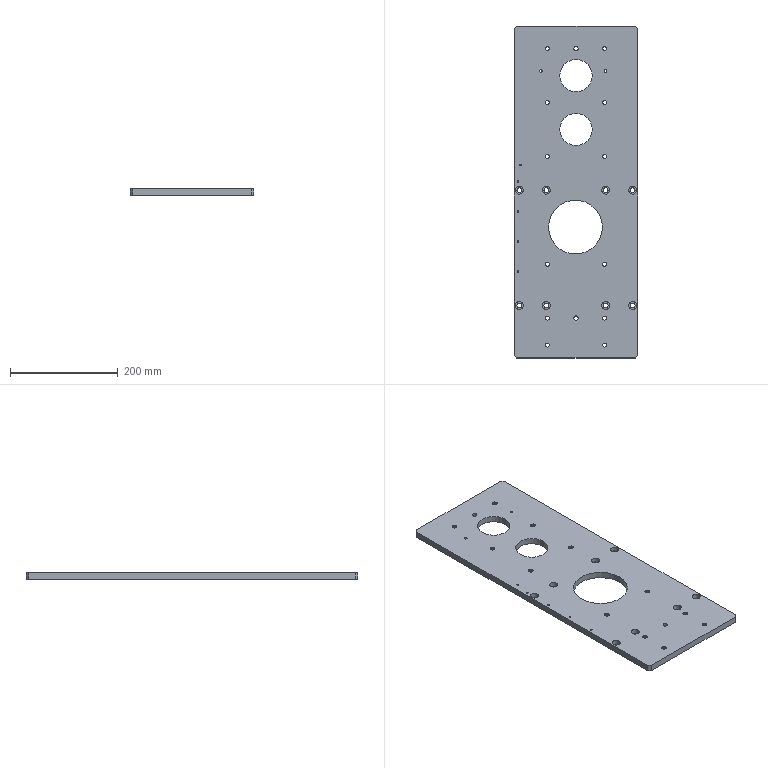Part | SolidWorks | features HoleWzd 6, Chamfer 1, Extrusion 1, ICE 1 | 1 solid | 158 faces | box 230 x 616 x 12 mm | volume 1500608 mm3 | cylinder 104 | plane 30 | cone 24 | commonest cylinder face diameters 9 x40 15 x40 3.3 x10 5 x4 8 x4 60 x4